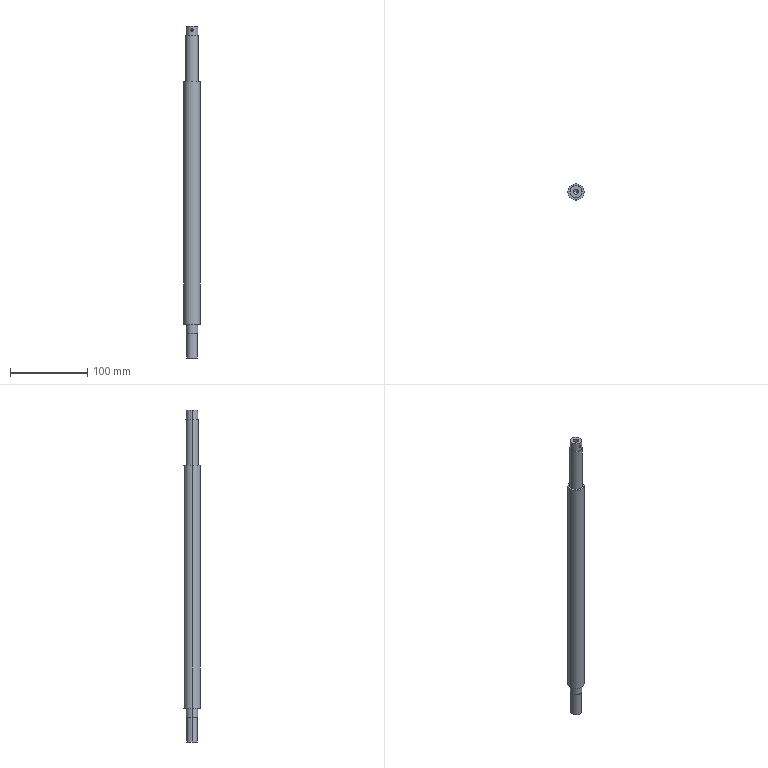Part | SolidWorks | features ICE 5, HoleWzd 2, 3DProfileFeature 1, Extrusion 1 | 1 solid | 28 faces | box 21 x 21 x 431 mm | volume 129224 mm3 | cylinder 16 | plane 10 | cone 2 | commonest cylinder face diameters 3.3 x4 15 x4 6.8 x2 14 x2 16 x2 21 x2
STEP:
#1=CARTESIAN_POINT('',(1.661,-7.314,6.663));
#2=VERTEX_POINT('',#1);
#3=CARTESIAN_POINT('',(-1.639,-7.319,6.663));
#4=VERTEX_POINT('',#3);
#5=CARTESIAN_POINT('',(1.661,-7.314,6.663));
#6=CARTESIAN_POINT('',(1.661,-7.314,6.448));
#7=CARTESIAN_POINT('',(1.617,-7.324,6.23));
#8=CARTESIAN_POINT('',(1.494,-7.35,5.932));
#9=CARTESIAN_POINT('',(1.442,-7.36,5.836));
#10=CARTESIAN_POINT('',(1.322,-7.383,5.656));
#11=CARTESIAN_POINT('',(1.254,-7.395,5.573));
#12=CARTESIAN_POINT('',(1.102,-7.419,5.421));
#13=CARTESIAN_POINT('',(1.018,-7.431,5.352));
#14=CARTESIAN_POINT('',(0.8393,-7.453,5.232));
#15=CARTESIAN_POINT('',(0.7447,-7.464,5.182));
#16=CARTESIAN_POINT('',(0.4441,-7.49,5.057));
#17=CARTESIAN_POINT('',(0.2295,-7.5,5.014));
#18=CARTESIAN_POINT('',(-0.09721,-7.5,5.013));
#19=CARTESIAN_POINT('',(-0.2045,-7.498,5.024));
#20=CARTESIAN_POINT('',(-0.4162,-7.489,5.066));
#21=CARTESIAN_POINT('',(-0.5215,-7.483,5.098));
#22=CARTESIAN_POINT('',(-0.8203,-7.458,5.222));
#23=CARTESIAN_POINT('',(-1.004,-7.434,5.345));
#24=CARTESIAN_POINT('',(-1.307,-7.387,5.647));
#25=CARTESIAN_POINT('',(-1.43,-7.363,5.831));
#26=CARTESIAN_POINT('',(-1.554,-7.337,6.129));
#27=CARTESIAN_POINT('',(-1.586,-7.33,6.233));
#28=CARTESIAN_POINT('',(-1.629,-7.321,6.446));
#29=CARTESIAN_POINT('',(-1.639,-7.319,6.554));
#30=CARTESIAN_POINT('',(-1.639,-7.319,6.663));
#31=B_SPLINE_CURVE_WITH_KNOTS('',3,(#5,#6,#7,#8,#9,#10,#11,#12,#13,#14,#15,#16,#17,#18,#19,#20,#21,#22,#23,#24,#25,#26,#27,#28,#29,#30),.UNSPECIFIED.,.F.,.F.,(4,2,2,2,2,2,2,2,2,2,2,2,4),(0.005174,0.005821,0.006144,0.006468,0.006791,0.007114,0.007761,0.008084,0.008408,0.009054,0.009701,0.01002,0.01035),.UNSPECIFIED.);
#32=EDGE_CURVE('',#2,#4,#31,.T.);
#33=ORIENTED_EDGE('',*,*,#32,.F.);
#34=CARTESIAN_POINT('',(1.654,-2.97,6.663));
#35=VERTEX_POINT('',#34);
#36=CARTESIAN_POINT('',(1.639,7.502,6.663));
#37=DIRECTION('',(-0.001464,1.,0.));
#38=VECTOR('',#37,1000.);
#39=LINE('',#36,#38);
#40=EDGE_CURVE('',#2,#35,#39,.T.);
#41=ORIENTED_EDGE('',*,*,#40,.T.);
#42=CARTESIAN_POINT('',(-1.646,-2.975,6.663));
#43=VERTEX_POINT('',#42);
#44=CARTESIAN_POINT('',(-1.646,-2.975,6.663));
#45=CARTESIAN_POINT('',(-1.646,-2.975,6.552));
#46=CARTESIAN_POINT('',(-1.635,-2.981,6.444));
#47=CARTESIAN_POINT('',(-1.592,-3.005,6.231));
#48=CARTESIAN_POINT('',(-1.559,-3.022,6.125));
#49=CARTESIAN_POINT('',(-1.434,-3.084,5.827));
#50=CARTESIAN_POINT('',(-1.312,-3.141,5.647));
#51=CARTESIAN_POINT('',(-1.013,-3.25,5.347));
#52=CARTESIAN_POINT('',(-0.8316,-3.303,5.225));
#53=CARTESIAN_POINT('',(-0.5341,-3.359,5.1));
#54=CARTESIAN_POINT('',(-0.4283,-3.375,5.068));
#55=CARTESIAN_POINT('',(-0.2142,-3.395,5.024));
#56=CARTESIAN_POINT('',(-0.1059,-3.4,5.013));
#57=CARTESIAN_POINT('',(0.1137,-3.4,5.013));
#58=CARTESIAN_POINT('',(0.2247,-3.394,5.025));
#59=CARTESIAN_POINT('',(0.4383,-3.373,5.068));
#60=CARTESIAN_POINT('',(0.543,-3.358,5.1));
#61=CARTESIAN_POINT('',(0.7435,-3.319,5.184));
#62=CARTESIAN_POINT('',(0.8377,-3.296,5.235));
#63=CARTESIAN_POINT('',(1.015,-3.246,5.355));
#64=CARTESIAN_POINT('',(1.098,-3.219,5.423));
#65=CARTESIAN_POINT('',(1.323,-3.136,5.649));
#66=CARTESIAN_POINT('',(1.444,-3.079,5.83));
#67=CARTESIAN_POINT('',(1.609,-2.996,6.225));
#68=CARTESIAN_POINT('',(1.654,-2.97,6.445));
#69=CARTESIAN_POINT('',(1.654,-2.97,6.663));
#70=B_SPLINE_CURVE_WITH_KNOTS('',3,(#44,#45,#46,#47,#48,#49,#50,#51,#52,#53,#54,#55,#56,#57,#58,#59,#60,#61,#62,#63,#64,#65,#66,#67,#68,#69),.UNSPECIFIED.,.F.,.F.,(4,2,2,2,2,2,2,2,2,2,2,2,4),(0.,0.0003276,0.0006553,0.001311,0.001966,0.002293,0.002621,0.002949,0.003276,0.003604,0.003932,0.004587,0.005242),.UNSPECIFIED.);
#71=EDGE_CURVE('',#43,#35,#70,.T.);
#72=ORIENTED_EDGE('',*,*,#71,.F.);
#73=CARTESIAN_POINT('',(-1.661,7.498,6.663));
#74=DIRECTION('',(-0.001464,1.,0.));
#75=VECTOR('',#74,1000.);
#76=LINE('',#73,#75);
#77=EDGE_CURVE('',#4,#43,#76,.T.);
#78=ORIENTED_EDGE('',*,*,#77,.F.);
#79=EDGE_LOOP('',(#33,#41,#72,#78));
#80=FACE_OUTER_BOUND('',#79,.T.);
#81=CARTESIAN_POINT('',(-0.01098,7.5,6.663));
#82=DIRECTION('',(-0.001464,1.,0.));
#83=DIRECTION('',(-1.,-0.001464,0.));
#84=AXIS2_PLACEMENT_3D('',#81,#82,#83);
#85=CYLINDRICAL_SURFACE('',#84,1.65);
#86=ADVANCED_FACE('',(#80),#85,.F.);
#87=CARTESIAN_POINT('',(1.646,2.975,6.663));
#88=VERTEX_POINT('',#87);
#89=CARTESIAN_POINT('',(-1.654,2.97,6.663));
#90=VERTEX_POINT('',#89);
#91=CARTESIAN_POINT('',(1.646,2.975,6.663));
#92=CARTESIAN_POINT('',(1.646,2.975,6.554));
#93=CARTESIAN_POINT('',(1.635,2.981,6.443));
#94=CARTESIAN_POINT('',(1.591,3.005,6.23));
#95=CARTESIAN_POINT('',(1.559,3.022,6.126));
#96=CARTESIAN_POINT('',(1.434,3.084,5.826));
#97=CARTESIAN_POINT('',(1.312,3.141,5.647));
#98=CARTESIAN_POINT('',(1.087,3.223,5.422));
#99=CARTESIAN_POINT('',(1.005,3.249,5.354));
#100=CARTESIAN_POINT('',(0.8279,3.299,5.235));
#101=CARTESIAN_POINT('',(0.7318,3.322,5.183));
#102=CARTESIAN_POINT('',(0.4346,3.378,5.059));
#103=CARTESIAN_POINT('',(0.2144,3.4,5.014));
#104=CARTESIAN_POINT('',(-0.1129,3.4,5.013));
#105=CARTESIAN_POINT('',(-0.2233,3.394,5.024));
#106=CARTESIAN_POINT('',(-0.4382,3.373,5.068));
#107=CARTESIAN_POINT('',(-0.5418,3.358,5.099));
#108=CARTESIAN_POINT('',(-0.8413,3.301,5.225));
#109=CARTESIAN_POINT('',(-1.021,3.247,5.346));
#110=CARTESIAN_POINT('',(-1.248,3.164,5.573));
#111=CARTESIAN_POINT('',(-1.315,3.136,5.655));
#112=CARTESIAN_POINT('',(-1.433,3.084,5.831));
#113=CARTESIAN_POINT('',(-1.485,3.059,5.927));
#114=CARTESIAN_POINT('',(-1.568,3.017,6.125));
#115=CARTESIAN_POINT('',(-1.6,3.,6.228));
#116=CARTESIAN_POINT('',(-1.643,2.977,6.441));
#117=CARTESIAN_POINT('',(-1.654,2.97,6.553));
#118=CARTESIAN_POINT('',(-1.654,2.97,6.663));
#119=B_SPLINE_CURVE_WITH_KNOTS('',3,(#91,#92,#93,#94,#95,#96,#97,#98,#99,#100,#101,#102,#103,#104,#105,#106,#107,#108,#109,#110,#111,#112,#113,#114,#115,#116,#117,#118),.UNSPECIFIED.,.F.,.F.,(4,2,2,2,2,2,2,2,2,2,2,2,2,4),(0.005242,0.005569,0.005896,0.006551,0.006878,0.007205,0.007859,0.008186,0.008514,0.009168,0.009495,0.009822,0.01015,0.01048),.UNSPECIFIED.);
#120=EDGE_CURVE('',#88,#90,#119,.T.);
#121=ORIENTED_EDGE('',*,*,#120,.F.);
#122=CARTESIAN_POINT('',(1.639,7.319,6.663));
#123=VERTEX_POINT('',#122);
#124=CARTESIAN_POINT('',(1.639,7.502,6.663));
#125=DIRECTION('',(-0.001464,1.,0.));
#126=VECTOR('',#125,1000.);
#127=LINE('',#124,#126);
#128=EDGE_CURVE('',#88,#123,#127,.T.);
#129=ORIENTED_EDGE('',*,*,#128,.T.);
#130=CARTESIAN_POINT('',(-1.661,7.314,6.663));
#131=VERTEX_POINT('',#130);
#132=CARTESIAN_POINT('',(-1.661,7.314,6.663));
#133=CARTESIAN_POINT('',(-1.661,7.314,6.554));
#134=CARTESIAN_POINT('',(-1.65,7.316,6.447));
#135=CARTESIAN_POINT('',(-1.608,7.326,6.235));
#136=CARTESIAN_POINT('',(-1.576,7.333,6.13));
#137=CARTESIAN_POINT('',(-1.493,7.35,5.931));
#138=CARTESIAN_POINT('',(-1.442,7.36,5.836));
#139=CARTESIAN_POINT('',(-1.323,7.383,5.657));
#140=CARTESIAN_POINT('',(-1.253,7.395,5.572));
#141=CARTESIAN_POINT('',(-1.026,7.431,5.345));
#142=CARTESIAN_POINT('',(-0.8421,7.455,5.222));
#143=CARTESIAN_POINT('',(-0.4452,7.489,5.057));
#144=CARTESIAN_POINT('',(-0.2276,7.5,5.014));
#145=CARTESIAN_POINT('',(0.09636,7.5,5.013));
#146=CARTESIAN_POINT('',(0.2061,7.498,5.024));
#147=CARTESIAN_POINT('',(0.418,7.489,5.067));
#148=CARTESIAN_POINT('',(0.521,7.483,5.098));
#149=CARTESIAN_POINT('',(0.8214,7.458,5.222));
#150=CARTESIAN_POINT('',(1.003,7.434,5.344));
#151=CARTESIAN_POINT('',(1.233,7.398,5.574));
#152=CARTESIAN_POINT('',(1.301,7.387,5.656));
#153=CARTESIAN_POINT('',(1.42,7.365,5.835));
#154=CARTESIAN_POINT('',(1.472,7.354,5.932));
#155=CARTESIAN_POINT('',(1.555,7.337,6.131));
#156=CARTESIAN_POINT('',(1.586,7.33,6.234));
#157=CARTESIAN_POINT('',(1.628,7.321,6.446));
#158=CARTESIAN_POINT('',(1.639,7.319,6.556));
#159=CARTESIAN_POINT('',(1.639,7.319,6.663));
#160=B_SPLINE_CURVE_WITH_KNOTS('',3,(#132,#133,#134,#135,#136,#137,#138,#139,#140,#141,#142,#143,#144,#145,#146,#147,#148,#149,#150,#151,#152,#153,#154,#155,#156,#157,#158,#159),.UNSPECIFIED.,.F.,.F.,(4,2,2,2,2,2,2,2,2,2,2,2,2,4),(0.,0.0003234,0.0006468,0.0009702,0.001294,0.00194,0.002587,0.002911,0.003234,0.003881,0.004204,0.004528,0.004851,0.005174),.UNSPECIFIED.);
#161=EDGE_CURVE('',#131,#123,#160,.T.);
#162=ORIENTED_EDGE('',*,*,#161,.F.);
#163=CARTESIAN_POINT('',(-1.661,7.498,6.663));
#164=DIRECTION('',(-0.001464,1.,0.));
#165=VECTOR('',#164,1000.);
#166=LINE('',#163,#165);
#167=EDGE_CURVE('',#90,#131,#166,.T.);
#168=ORIENTED_EDGE('',*,*,#167,.F.);
#169=EDGE_LOOP('',(#121,#129,#162,#168));
#170=FACE_OUTER_BOUND('',#169,.T.);
#171=CARTESIAN_POINT('',(-0.01098,7.5,6.663));
#172=DIRECTION('',(-0.001464,1.,0.));
#173=DIRECTION('',(-1.,-0.001464,0.));
#174=AXIS2_PLACEMENT_3D('',#171,#172,#173);
#175=CYLINDRICAL_SURFACE('',#174,1.65);
#176=ADVANCED_FACE('',(#170),#175,.F.);
#177=ORIENTED_EDGE('',*,*,#71,.T.);
#178=CARTESIAN_POINT('',(1.654,-2.97,6.663));
#179=CARTESIAN_POINT('',(1.654,-2.97,6.773));
#180=CARTESIAN_POINT('',(1.643,-2.977,6.884));
#181=CARTESIAN_POINT('',(1.6,-3.,7.097));
#182=CARTESIAN_POINT('',(1.568,-3.017,7.201));
#183=CARTESIAN_POINT('',(1.443,-3.08,7.501));
#184=CARTESIAN_POINT('',(1.321,-3.137,7.68));
#185=CARTESIAN_POINT('',(1.096,-3.219,7.905));
#186=CARTESIAN_POINT('',(1.015,-3.246,7.973));
#187=CARTESIAN_POINT('',(0.8375,-3.297,8.092));
#188=CARTESIAN_POINT('',(0.7416,-3.32,8.144));
#189=CARTESIAN_POINT('',(0.4444,-3.377,8.268));
#190=CARTESIAN_POINT('',(0.2244,-3.4,8.313));
#191=CARTESIAN_POINT('',(-0.1029,-3.4,8.314));
#192=CARTESIAN_POINT('',(-0.2134,-3.395,8.303));
#193=CARTESIAN_POINT('',(-0.4284,-3.375,8.259));
#194=CARTESIAN_POINT('',(-0.5319,-3.36,8.227));
#195=CARTESIAN_POINT('',(-0.8317,-3.303,8.102));
#196=CARTESIAN_POINT('',(-1.012,-3.25,7.981));
#197=CARTESIAN_POINT('',(-1.238,-3.167,7.754));
#198=CARTESIAN_POINT('',(-1.306,-3.14,7.672));
#199=CARTESIAN_POINT('',(-1.424,-3.088,7.496));
#200=CARTESIAN_POINT('',(-1.476,-3.063,7.4));
#201=CARTESIAN_POINT('',(-1.559,-3.022,7.201));
#202=CARTESIAN_POINT('',(-1.591,-3.005,7.099));
#203=CARTESIAN_POINT('',(-1.634,-2.982,6.885));
#204=CARTESIAN_POINT('',(-1.646,-2.975,6.774));
#205=CARTESIAN_POINT('',(-1.646,-2.975,6.663));
#206=B_SPLINE_CURVE_WITH_KNOTS('',3,(#178,#179,#180,#181,#182,#183,#184,#185,#186,#187,#188,#189,#190,#191,#192,#193,#194,#195,#196,#197,#198,#199,#200,#201,#202,#203,#204,#205),.UNSPECIFIED.,.F.,.F.,(4,2,2,2,2,2,2,2,2,2,2,2,2,4),(0.005242,0.005569,0.005896,0.006551,0.006878,0.007205,0.007859,0.008186,0.008514,0.009168,0.009495,0.009822,0.01015,0.01048),.UNSPECIFIED.);
#207=EDGE_CURVE('',#35,#43,#206,.T.);
#208=ORIENTED_EDGE('',*,*,#207,.T.);
#209=EDGE_LOOP('',(#177,#208));
#210=FACE_BOUND('',#209,.T.);
#211=CARTESIAN_POINT('',(-3.4,0.,-7.75));
#212=VERTEX_POINT('',#211);
#213=CARTESIAN_POINT('',(3.4,0.,-7.75));
#214=VERTEX_POINT('',#213);
#215=CARTESIAN_POINT('',(0.,0.,-7.75));
#216=DIRECTION('',(0.,0.,1.));
#217=DIRECTION('',(1.,0.,0.));
#218=AXIS2_PLACEMENT_3D('',#215,#216,#217);
#219=CIRCLE('',#218,3.4);
#220=EDGE_CURVE('',#212,#214,#219,.T.);
#221=ORIENTED_EDGE('',*,*,#220,.F.);
#222=CARTESIAN_POINT('',(-3.4,0.,12.));
#223=VERTEX_POINT('',#222);
#224=CARTESIAN_POINT('',(-3.4,0.,12.));
#225=DIRECTION('',(0.,0.,1.));
#226=VECTOR('',#225,1000.);
#227=LINE('',#224,#226);
#228=EDGE_CURVE('',#212,#223,#227,.T.);
#229=ORIENTED_EDGE('',*,*,#228,.T.);
#230=CARTESIAN_POINT('',(3.4,0.,12.));
#231=VERTEX_POINT('',#230);
#232=CARTESIAN_POINT('',(0.,0.,12.));
#233=DIRECTION('',(0.,0.,1.));
#234=DIRECTION('',(1.,0.,0.));
#235=AXIS2_PLACEMENT_3D('',#232,#233,#234);
#236=CIRCLE('',#235,3.4);
#237=EDGE_CURVE('',#223,#231,#236,.T.);
#238=ORIENTED_EDGE('',*,*,#237,.T.);
#239=CARTESIAN_POINT('',(3.4,0.,12.));
#240=DIRECTION('',(0.,0.,1.));
#241=VECTOR('',#240,1000.);
#242=LINE('',#239,#241);
#243=EDGE_CURVE('',#214,#231,#242,.T.);
#244=ORIENTED_EDGE('',*,*,#243,.F.);
#245=EDGE_LOOP('',(#221,#229,#238,#244));
#246=FACE_OUTER_BOUND('',#245,.T.);
#247=CARTESIAN_POINT('',(0.,0.,12.));
#248=DIRECTION('',(0.,0.,1.));
#249=DIRECTION('',(1.,0.,0.));
#250=AXIS2_PLACEMENT_3D('',#247,#248,#249);
#251=CYLINDRICAL_SURFACE('',#250,3.4);
#252=ADVANCED_FACE('',(#210,#246),#251,.F.);
#253=CARTESIAN_POINT('',(0.,0.,-9.793));
#254=VERTEX_POINT('',#253);
#255=CARTESIAN_POINT('',(3.4,0.,-7.75));
#256=DIRECTION('',(0.8572,0.,0.515));
#257=VECTOR('',#256,1000.);
#258=LINE('',#255,#257);
#259=EDGE_CURVE('',#254,#214,#258,.T.);
#260=ORIENTED_EDGE('',*,*,#259,.F.);
#261=CARTESIAN_POINT('',(-3.4,0.,-7.75));
#262=DIRECTION('',(-0.8572,0.,0.515));
#263=VECTOR('',#262,1000.);
#264=LINE('',#261,#263);
#265=EDGE_CURVE('',#254,#212,#264,.T.);
#266=ORIENTED_EDGE('',*,*,#265,.T.);
#267=ORIENTED_EDGE('',*,*,#220,.T.);
#268=EDGE_LOOP('',(#260,#266,#267));
#269=FACE_OUTER_BOUND('',#268,.T.);
#270=CARTESIAN_POINT('',(0.,0.,-7.75));
#271=DIRECTION('',(0.,0.,1.));
#272=DIRECTION('',(1.,0.,0.));
#273=AXIS2_PLACEMENT_3D('',#270,#271,#272);
#274=CONICAL_SURFACE('',#273,3.4,1.03);
#275=ADVANCED_FACE('',(#269),#274,.F.);
#276=CARTESIAN_POINT('',(-7.,0.,-419.));
#277=VERTEX_POINT('',#276);
#278=CARTESIAN_POINT('',(-2.354,6.592,-419.));
#279=VERTEX_POINT('',#278);
#280=CARTESIAN_POINT('',(0.,0.,-419.));
#281=DIRECTION('',(0.,0.,-1.));
#282=DIRECTION('',(-1.,0.,0.));
#283=AXIS2_PLACEMENT_3D('',#280,#281,#282);
#284=CIRCLE('',#283,7.);
#285=EDGE_CURVE('',#277,#279,#284,.T.);
#286=ORIENTED_EDGE('',*,*,#285,.F.);
#287=CARTESIAN_POINT('',(-7.,0.,-387.));
#288=VERTEX_POINT('',#287);
#289=CARTESIAN_POINT('',(-7.,0.,-419.));
#290=DIRECTION('',(0.,0.,1.));
#291=VECTOR('',#290,1000.);
#292=LINE('',#289,#291);
#293=EDGE_CURVE('',#277,#288,#292,.T.);
#294=ORIENTED_EDGE('',*,*,#293,.T.);
#295=CARTESIAN_POINT('',(7.,0.,-387.));
#296=VERTEX_POINT('',#295);
#297=CARTESIAN_POINT('',(0.,0.,-387.));
#298=DIRECTION('',(0.,0.,-1.));
#299=DIRECTION('',(-1.,0.,0.));
#300=AXIS2_PLACEMENT_3D('',#297,#298,#299);
#301=CIRCLE('',#300,7.);
#302=EDGE_CURVE('',#288,#296,#301,.T.);
#303=ORIENTED_EDGE('',*,*,#302,.T.);
#304=CARTESIAN_POINT('',(7.,0.,-419.));
#305=VERTEX_POINT('',#304);
#306=CARTESIAN_POINT('',(7.,0.,-419.));
#307=DIRECTION('',(0.,0.,1.));
#308=VECTOR('',#307,1000.);
#309=LINE('',#306,#308);
#310=EDGE_CURVE('',#305,#296,#309,.T.);
#311=ORIENTED_EDGE('',*,*,#310,.F.);
#312=CARTESIAN_POINT('',(2.354,6.592,-419.));
#313=VERTEX_POINT('',#312);
#314=CARTESIAN_POINT('',(0.,0.,-419.));
#315=DIRECTION('',(0.,0.,-1.));
#316=DIRECTION('',(-1.,0.,0.));
#317=AXIS2_PLACEMENT_3D('',#314,#315,#316);
#318=CIRCLE('',#317,7.);
#319=EDGE_CURVE('',#313,#305,#318,.T.);
#320=ORIENTED_EDGE('',*,*,#319,.F.);
#321=CARTESIAN_POINT('',(2.354,6.592,-389.));
#322=VERTEX_POINT('',#321);
#323=CARTESIAN_POINT('',(2.354,6.592,-419.));
#324=DIRECTION('',(0.,0.,1.));
#325=VECTOR('',#324,1000.);
#326=LINE('',#323,#325);
#327=EDGE_CURVE('',#313,#322,#326,.T.);
#328=ORIENTED_EDGE('',*,*,#327,.T.);
#329=CARTESIAN_POINT('',(-2.354,6.592,-389.));
#330=VERTEX_POINT('',#329);
#331=CARTESIAN_POINT('',(0.,0.,-389.));
#332=DIRECTION('',(0.,0.,1.));
#333=DIRECTION('',(1.,0.,0.));
#334=AXIS2_PLACEMENT_3D('',#331,#332,#333);
#335=CIRCLE('',#334,7.);
#336=EDGE_CURVE('',#322,#330,#335,.T.);
#337=ORIENTED_EDGE('',*,*,#336,.T.);
#338=CARTESIAN_POINT('',(-2.354,6.592,-419.));
#339=DIRECTION('',(0.,0.,-1.));
#340=VECTOR('',#339,1000.);
#341=LINE('',#338,#340);
#342=EDGE_CURVE('',#330,#279,#341,.T.);
#343=ORIENTED_EDGE('',*,*,#342,.T.);
#344=EDGE_LOOP('',(#286,#294,#303,#311,#320,#328,#337,#343));
#345=FACE_OUTER_BOUND('',#344,.T.);
#346=CARTESIAN_POINT('',(0.,0.,-419.));
#347=DIRECTION('',(0.,0.,1.));
#348=DIRECTION('',(1.,0.,0.));
#349=AXIS2_PLACEMENT_3D('',#346,#347,#348);
#350=CYLINDRICAL_SURFACE('',#349,7.);
#351=ADVANCED_FACE('',(#345),#350,.T.);
#352=CARTESIAN_POINT('',(-7.5,0.,-387.));
#353=VERTEX_POINT('',#352);
#354=CARTESIAN_POINT('',(7.5,0.,-387.));
#355=VERTEX_POINT('',#354);
#356=CARTESIAN_POINT('',(0.,0.,-387.));
#357=DIRECTION('',(0.,0.,-1.));
#358=DIRECTION('',(-1.,0.,0.));
#359=AXIS2_PLACEMENT_3D('',#356,#357,#358);
#360=CIRCLE('',#359,7.5);
#361=EDGE_CURVE('',#353,#355,#360,.T.);
#362=ORIENTED_EDGE('',*,*,#361,.F.);
#363=CARTESIAN_POINT('',(-7.5,0.,-375.));
#364=VERTEX_POINT('',#363);
#365=CARTESIAN_POINT('',(-7.5,0.,-387.));
#366=DIRECTION('',(0.,0.,1.));
#367=VECTOR('',#366,1000.);
#368=LINE('',#365,#367);
#369=EDGE_CURVE('',#353,#364,#368,.T.);
#370=ORIENTED_EDGE('',*,*,#369,.T.);
#371=CARTESIAN_POINT('',(7.5,0.,-375.));
#372=VERTEX_POINT('',#371);
#373=CARTESIAN_POINT('',(0.,0.,-375.));
#374=DIRECTION('',(0.,0.,-1.));
#375=DIRECTION('',(-1.,0.,0.));
#376=AXIS2_PLACEMENT_3D('',#373,#374,#375);
#377=CIRCLE('',#376,7.5);
#378=EDGE_CURVE('',#364,#372,#377,.T.);
#379=ORIENTED_EDGE('',*,*,#378,.T.);
#380=CARTESIAN_POINT('',(7.5,0.,-387.));
#381=DIRECTION('',(0.,0.,1.));
#382=VECTOR('',#381,1000.);
#383=LINE('',#380,#382);
#384=EDGE_CURVE('',#355,#372,#383,.T.);
#385=ORIENTED_EDGE('',*,*,#384,.F.);
#386=EDGE_LOOP('',(#362,#370,#379,#385));
#387=FACE_OUTER_BOUND('',#386,.T.);
#388=CARTESIAN_POINT('',(0.,0.,-387.));
#389=DIRECTION('',(0.,0.,1.));
#390=DIRECTION('',(1.,0.,0.));
#391=AXIS2_PLACEMENT_3D('',#388,#389,#390);
#392=CYLINDRICAL_SURFACE('',#391,7.5);
#393=ADVANCED_FACE('',(#387),#392,.T.);
#394=CARTESIAN_POINT('',(-10.5,0.,-375.));
#395=VERTEX_POINT('',#394);
#396=CARTESIAN_POINT('',(10.5,0.,-375.));
#397=VERTEX_POINT('',#396);
#398=CARTESIAN_POINT('',(0.,0.,-375.));
#399=DIRECTION('',(0.,0.,-1.));
#400=DIRECTION('',(-1.,0.,0.));
#401=AXIS2_PLACEMENT_3D('',#398,#399,#400);
#402=CIRCLE('',#401,10.5);
#403=EDGE_CURVE('',#395,#397,#402,.T.);
#404=ORIENTED_EDGE('',*,*,#403,.F.);
#405=CARTESIAN_POINT('',(-10.5,0.,-60.));
#406=VERTEX_POINT('',#405);
#407=CARTESIAN_POINT('',(-10.5,0.,-375.));
#408=DIRECTION('',(0.,0.,1.));
#409=VECTOR('',#408,1000.);
#410=LINE('',#407,#409);
#411=EDGE_CURVE('',#395,#406,#410,.T.);
#412=ORIENTED_EDGE('',*,*,#411,.T.);
#413=CARTESIAN_POINT('',(10.5,0.,-60.));
#414=VERTEX_POINT('',#413);
#415=CARTESIAN_POINT('',(0.,0.,-60.));
#416=DIRECTION('',(0.,0.,-1.));
#417=DIRECTION('',(-1.,0.,0.));
#418=AXIS2_PLACEMENT_3D('',#415,#416,#417);
#419=CIRCLE('',#418,10.5);
#420=EDGE_CURVE('',#406,#414,#419,.T.);
#421=ORIENTED_EDGE('',*,*,#420,.T.);
#422=CARTESIAN_POINT('',(10.5,0.,-375.));
#423=DIRECTION('',(0.,0.,1.));
#424=VECTOR('',#423,1000.);
#425=LINE('',#422,#424);
#426=EDGE_CURVE('',#397,#414,#425,.T.);
#427=ORIENTED_EDGE('',*,*,#426,.F.);
#428=EDGE_LOOP('',(#404,#412,#421,#427));
#429=FACE_OUTER_BOUND('',#428,.T.);
#430=CARTESIAN_POINT('',(0.,0.,-375.));
#431=DIRECTION('',(0.,0.,1.));
#432=DIRECTION('',(1.,0.,0.));
#433=AXIS2_PLACEMENT_3D('',#430,#431,#432);
#434=CYLINDRICAL_SURFACE('',#433,10.5);
#435=ADVANCED_FACE('',(#429),#434,.T.);
#436=CARTESIAN_POINT('',(-8.,0.,-60.));
#437=VERTEX_POINT('',#436);
#438=CARTESIAN_POINT('',(8.,0.,-60.));
#439=VERTEX_POINT('',#438);
#440=CARTESIAN_POINT('',(0.,0.,-60.));
#441=DIRECTION('',(0.,0.,-1.));
#442=DIRECTION('',(-1.,0.,0.));
#443=AXIS2_PLACEMENT_3D('',#440,#441,#442);
#444=CIRCLE('',#443,8.);
#445=EDGE_CURVE('',#437,#439,#444,.T.);
#446=ORIENTED_EDGE('',*,*,#445,.F.);
#447=CARTESIAN_POINT('',(-8.,0.,0.));
#448=VERTEX_POINT('',#447);
#449=CARTESIAN_POINT('',(-8.,0.,-60.));
#450=DIRECTION('',(0.,0.,1.));
#451=VECTOR('',#450,1000.);
#452=LINE('',#449,#451);
#453=EDGE_CURVE('',#437,#448,#452,.T.);
#454=ORIENTED_EDGE('',*,*,#453,.T.);
#455=CARTESIAN_POINT('',(8.,0.,0.));
#456=VERTEX_POINT('',#455);
#457=CARTESIAN_POINT('',(0.,0.,0.));
#458=DIRECTION('',(0.,0.,-1.));
#459=DIRECTION('',(-1.,0.,0.));
#460=AXIS2_PLACEMENT_3D('',#457,#458,#459);
#461=CIRCLE('',#460,8.);
#462=EDGE_CURVE('',#448,#456,#461,.T.);
#463=ORIENTED_EDGE('',*,*,#462,.T.);
#464=CARTESIAN_POINT('',(8.,0.,-60.));
#465=DIRECTION('',(0.,0.,1.));
#466=VECTOR('',#465,1000.);
#467=LINE('',#464,#466);
#468=EDGE_CURVE('',#439,#456,#467,.T.);
#469=ORIENTED_EDGE('',*,*,#468,.F.);
#470=EDGE_LOOP('',(#446,#454,#463,#469));
#471=FACE_OUTER_BOUND('',#470,.T.);
#472=CARTESIAN_POINT('',(0.,0.,-60.));
#473=DIRECTION('',(0.,0.,1.));
#474=DIRECTION('',(1.,0.,0.));
#475=AXIS2_PLACEMENT_3D('',#472,#473,#474);
#476=CYLINDRICAL_SURFACE('',#475,8.);
#477=ADVANCED_FACE('',(#471),#476,.T.);
#478=ORIENTED_EDGE('',*,*,#161,.T.);
#479=CARTESIAN_POINT('',(1.639,7.319,6.663));
#480=CARTESIAN_POINT('',(1.639,7.319,6.879));
#481=CARTESIAN_POINT('',(1.596,7.329,7.097));
#482=CARTESIAN_POINT('',(1.472,7.354,7.395));
#483=CARTESIAN_POINT('',(1.421,7.364,7.491));
#484=CARTESIAN_POINT('',(1.301,7.387,7.671));
#485=CARTESIAN_POINT('',(1.233,7.398,7.753));
#486=CARTESIAN_POINT('',(1.081,7.422,7.906));
#487=CARTESIAN_POINT('',(0.9959,7.434,7.975));
#488=CARTESIAN_POINT('',(0.8174,7.456,8.094));
#489=CARTESIAN_POINT('',(0.7228,7.466,8.145));
#490=CARTESIAN_POINT('',(0.4222,7.491,8.27));
#491=CARTESIAN_POINT('',(0.2075,7.5,8.313));
#492=CARTESIAN_POINT('',(-0.1192,7.5,8.313));
#493=CARTESIAN_POINT('',(-0.2265,7.497,8.303));
#494=CARTESIAN_POINT('',(-0.4381,7.488,8.261));
#495=CARTESIAN_POINT('',(-0.5434,7.481,8.229));
#496=CARTESIAN_POINT('',(-0.8421,7.455,8.105));
#497=CARTESIAN_POINT('',(-1.025,7.431,7.982));
#498=CARTESIAN_POINT('',(-1.329,7.383,7.679));
#499=CARTESIAN_POINT('',(-1.451,7.359,7.496));
#500=CARTESIAN_POINT('',(-1.575,7.333,7.198));
#501=CARTESIAN_POINT('',(-1.607,7.326,7.093));
#502=CARTESIAN_POINT('',(-1.65,7.316,6.881));
#503=CARTESIAN_POINT('',(-1.661,7.314,6.773));
#504=CARTESIAN_POINT('',(-1.661,7.314,6.663));
#505=B_SPLINE_CURVE_WITH_KNOTS('',3,(#479,#480,#481,#482,#483,#484,#485,#486,#487,#488,#489,#490,#491,#492,#493,#494,#495,#496,#497,#498,#499,#500,#501,#502,#503,#504),.UNSPECIFIED.,.F.,.F.,(4,2,2,2,2,2,2,2,2,2,2,2,4),(0.005174,0.005821,0.006144,0.006468,0.006791,0.007114,0.007761,0.008084,0.008408,0.009054,0.009701,0.01002,0.01035),.UNSPECIFIED.);
#506=EDGE_CURVE('',#123,#131,#505,.T.);
#507=ORIENTED_EDGE('',*,*,#506,.T.);
#508=EDGE_LOOP('',(#478,#507));
#509=FACE_BOUND('',#508,.T.);
#510=CARTESIAN_POINT('',(7.5,0.,12.));
#511=VERTEX_POINT('',#510);
#512=CARTESIAN_POINT('',(-7.5,0.,12.));
#513=VERTEX_POINT('',#512);
#514=CARTESIAN_POINT('',(0.,0.,12.));
#515=DIRECTION('',(0.,0.,1.));
#516=DIRECTION('',(1.,0.,0.));
#517=AXIS2_PLACEMENT_3D('',#514,#515,#516);
#518=CIRCLE('',#517,7.5);
#519=EDGE_CURVE('',#511,#513,#518,.T.);
#520=ORIENTED_EDGE('',*,*,#519,.F.);
#521=CARTESIAN_POINT('',(7.5,0.,0.));
#522=VERTEX_POINT('',#521);
#523=CARTESIAN_POINT('',(7.5,0.,12.));
#524=DIRECTION('',(0.,0.,-1.));
#525=VECTOR('',#524,1000.);
#526=LINE('',#523,#525);
#527=EDGE_CURVE('',#511,#522,#526,.T.);
#528=ORIENTED_EDGE('',*,*,#527,.T.);
#529=CARTESIAN_POINT('',(-7.5,0.,0.));
#530=VERTEX_POINT('',#529);
#531=CARTESIAN_POINT('',(0.,0.,0.));
#532=DIRECTION('',(0.,0.,-1.));
#533=DIRECTION('',(-1.,0.,0.));
#534=AXIS2_PLACEMENT_3D('',#531,#532,#533);
#535=CIRCLE('',#534,7.5);
#536=EDGE_CURVE('',#530,#522,#535,.T.);
#537=ORIENTED_EDGE('',*,*,#536,.F.);
#538=CARTESIAN_POINT('',(-7.5,0.,12.));
#539=DIRECTION('',(0.,0.,-1.));
#540=VECTOR('',#539,1000.);
#541=LINE('',#538,#540);
#542=EDGE_CURVE('',#513,#530,#541,.T.);
#543=ORIENTED_EDGE('',*,*,#542,.F.);
#544=EDGE_LOOP('',(#520,#528,#537,#543));
#545=FACE_OUTER_BOUND('',#544,.T.);
#546=CARTESIAN_POINT('',(0.,0.,12.));
#547=DIRECTION('',(0.,0.,-1.));
#548=DIRECTION('',(-1.,0.,0.));
#549=AXIS2_PLACEMENT_3D('',#546,#547,#548);
#550=CYLINDRICAL_SURFACE('',#549,7.5);
#551=ADVANCED_FACE('',(#509,#545),#550,.T.);
#552=CARTESIAN_POINT('',(0.,0.,-387.));
#553=DIRECTION('',(0.,0.,-1.));
#554=DIRECTION('',(-1.,0.,0.));
#555=AXIS2_PLACEMENT_3D('',#552,#553,#554);
#556=CIRCLE('',#555,7.5);
#557=EDGE_CURVE('',#355,#353,#556,.T.);
#558=ORIENTED_EDGE('',*,*,#557,.T.);
#559=ORIENTED_EDGE('',*,*,#361,.T.);
#560=EDGE_LOOP('',(#558,#559));
#561=FACE_OUTER_BOUND('',#560,.T.);
#562=CARTESIAN_POINT('',(0.,0.,-387.));
#563=DIRECTION('',(0.,0.,-1.));
#564=DIRECTION('',(-1.,0.,0.));
#565=AXIS2_PLACEMENT_3D('',#562,#563,#564);
#566=CIRCLE('',#565,7.);
#567=EDGE_CURVE('',#296,#288,#566,.T.);
#568=ORIENTED_EDGE('',*,*,#567,.F.);
#569=ORIENTED_EDGE('',*,*,#302,.F.);
#570=EDGE_LOOP('',(#568,#569));
#571=FACE_BOUND('',#570,.T.);
#572=CARTESIAN_POINT('',(0.,0.,-387.));
#573=DIRECTION('',(0.,0.,-1.));
#574=DIRECTION('',(-1.,0.,0.));
#575=AXIS2_PLACEMENT_3D('',#572,#573,#574);
#576=PLANE('',#575);
#577=ADVANCED_FACE('',(#561,#571),#576,.T.);
#578=CARTESIAN_POINT('',(0.,0.,-375.));
#579=DIRECTION('',(0.,0.,-1.));
#580=DIRECTION('',(-1.,0.,0.));
#581=AXIS2_PLACEMENT_3D('',#578,#579,#580);
#582=CIRCLE('',#581,10.5);
#583=EDGE_CURVE('',#397,#395,#582,.T.);
#584=ORIENTED_EDGE('',*,*,#583,.T.);
#585=ORIENTED_EDGE('',*,*,#403,.T.);
#586=EDGE_LOOP('',(#584,#585));
#587=FACE_OUTER_BOUND('',#586,.T.);
#588=CARTESIAN_POINT('',(0.,0.,-375.));
#589=DIRECTION('',(0.,0.,-1.));
#590=DIRECTION('',(-1.,0.,0.));
#591=AXIS2_PLACEMENT_3D('',#588,#589,#590);
#592=CIRCLE('',#591,7.5);
#593=EDGE_CURVE('',#372,#364,#592,.T.);
#594=ORIENTED_EDGE('',*,*,#593,.F.);
#595=ORIENTED_EDGE('',*,*,#378,.F.);
#596=EDGE_LOOP('',(#594,#595));
#597=FACE_BOUND('',#596,.T.);
#598=CARTESIAN_POINT('',(0.,0.,-375.));
#599=DIRECTION('',(0.,0.,-1.));
#600=DIRECTION('',(-1.,0.,0.));
#601=AXIS2_PLACEMENT_3D('',#598,#599,#600);
#602=PLANE('',#601);
#603=ADVANCED_FACE('',(#587,#597),#602,.T.);
#604=ORIENTED_EDGE('',*,*,#527,.F.);
#605=CARTESIAN_POINT('',(0.,0.,12.));
#606=DIRECTION('',(0.,0.,1.));
#607=DIRECTION('',(1.,0.,0.));
#608=AXIS2_PLACEMENT_3D('',#605,#606,#607);
#609=CIRCLE('',#608,7.5);
#610=EDGE_CURVE('',#513,#511,#609,.T.);
#611=ORIENTED_EDGE('',*,*,#610,.F.);
#612=ORIENTED_EDGE('',*,*,#542,.T.);
#613=CARTESIAN_POINT('',(0.,0.,0.));
#614=DIRECTION('',(0.,0.,-1.));
#615=DIRECTION('',(-1.,0.,0.));
#616=AXIS2_PLACEMENT_3D('',#613,#614,#615);
#617=CIRCLE('',#616,7.5);
#618=EDGE_CURVE('',#522,#530,#617,.T.);
#619=ORIENTED_EDGE('',*,*,#618,.F.);
#620=EDGE_LOOP('',(#604,#611,#612,#619));
#621=FACE_OUTER_BOUND('',#620,.T.);
#622=CARTESIAN_POINT('',(-1.639,-7.319,6.663));
#623=CARTESIAN_POINT('',(-1.639,-7.319,6.773));
#624=CARTESIAN_POINT('',(-1.629,-7.321,6.88));
#625=CARTESIAN_POINT('',(-1.586,-7.33,7.092));
#626=CARTESIAN_POINT('',(-1.554,-7.337,7.197));
#627=CARTESIAN_POINT('',(-1.471,-7.354,7.396));
#628=CARTESIAN_POINT('',(-1.421,-7.364,7.491));
#629=CARTESIAN_POINT('',(-1.301,-7.387,7.67));
#630=CARTESIAN_POINT('',(-1.232,-7.399,7.755));
#631=CARTESIAN_POINT('',(-1.004,-7.434,7.982));
#632=CARTESIAN_POINT('',(-0.8202,-7.458,8.105));
#633=CARTESIAN_POINT('',(-0.4233,-7.491,8.27));
#634=CARTESIAN_POINT('',(-0.2057,-7.5,8.313));
#635=CARTESIAN_POINT('',(0.1183,-7.5,8.313));
#636=CARTESIAN_POINT('',(0.228,-7.497,8.303));
#637=CARTESIAN_POINT('',(0.4399,-7.488,8.26));
#638=CARTESIAN_POINT('',(0.5429,-7.481,8.229));
#639=CARTESIAN_POINT('',(0.8432,-7.455,8.105));
#640=CARTESIAN_POINT('',(1.025,-7.431,7.983));
#641=CARTESIAN_POINT('',(1.254,-7.395,7.753));
#642=CARTESIAN_POINT('',(1.322,-7.383,7.67));
#643=CARTESIAN_POINT('',(1.442,-7.36,7.492));
#644=CARTESIAN_POINT('',(1.494,-7.35,7.395));
#645=CARTESIAN_POINT('',(1.576,-7.333,7.196));
#646=CARTESIAN_POINT('',(1.607,-7.326,7.093));
#647=CARTESIAN_POINT('',(1.65,-7.316,6.881));
#648=CARTESIAN_POINT('',(1.661,-7.314,6.771));
#649=CARTESIAN_POINT('',(1.661,-7.314,6.663));
#650=B_SPLINE_CURVE_WITH_KNOTS('',3,(#622,#623,#624,#625,#626,#627,#628,#629,#630,#631,#632,#633,#634,#635,#636,#637,#638,#639,#640,#641,#642,#643,#644,#645,#646,#647,#648,#649),.UNSPECIFIED.,.F.,.F.,(4,2,2,2,2,2,2,2,2,2,2,2,2,4),(0.,0.0003234,0.0006468,0.0009702,0.001294,0.00194,0.002587,0.002911,0.003234,0.003881,0.004204,0.004528,0.004851,0.005174),.UNSPECIFIED.);
#651=EDGE_CURVE('',#4,#2,#650,.T.);
#652=ORIENTED_EDGE('',*,*,#651,.T.);
#653=ORIENTED_EDGE('',*,*,#32,.T.);
#654=EDGE_LOOP('',(#652,#653));
#655=FACE_BOUND('',#654,.T.);
#656=CARTESIAN_POINT('',(0.,0.,12.));
#657=DIRECTION('',(0.,0.,-1.));
#658=DIRECTION('',(-1.,0.,0.));
#659=AXIS2_PLACEMENT_3D('',#656,#657,#658);
#660=CYLINDRICAL_SURFACE('',#659,7.5);
#661=ADVANCED_FACE('',(#621,#655),#660,.T.);
#662=CARTESIAN_POINT('',(0.,0.,12.));
#663=DIRECTION('',(0.,0.,1.));
#664=DIRECTION('',(1.,0.,0.));
#665=AXIS2_PLACEMENT_3D('',#662,#663,#664);
#666=CIRCLE('',#665,3.4);
#667=EDGE_CURVE('',#231,#223,#666,.T.);
#668=ORIENTED_EDGE('',*,*,#667,.F.);
#669=ORIENTED_EDGE('',*,*,#237,.F.);
#670=EDGE_LOOP('',(#668,#669));
#671=FACE_BOUND('',#670,.T.);
#672=ORIENTED_EDGE('',*,*,#610,.T.);
#673=ORIENTED_EDGE('',*,*,#519,.T.);
#674=EDGE_LOOP('',(#672,#673));
#675=FACE_OUTER_BOUND('',#674,.T.);
#676=CARTESIAN_POINT('',(0.,0.,12.));
#677=DIRECTION('',(0.,0.,1.));
#678=DIRECTION('',(1.,0.,0.));
#679=AXIS2_PLACEMENT_3D('',#676,#677,#678);
#680=PLANE('',#679);
#681=ADVANCED_FACE('',(#671,#675),#680,.T.);
#682=CARTESIAN_POINT('',(0.,0.,0.));
#683=DIRECTION('',(0.,0.,-1.));
#684=DIRECTION('',(-1.,0.,0.));
#685=AXIS2_PLACEMENT_3D('',#682,#683,#684);
#686=CIRCLE('',#685,8.);
#687=EDGE_CURVE('',#456,#448,#686,.T.);
#688=ORIENTED_EDGE('',*,*,#687,.F.);
#689=ORIENTED_EDGE('',*,*,#462,.F.);
#690=EDGE_LOOP('',(#688,#689));
#691=FACE_OUTER_BOUND('',#690,.T.);
#692=ORIENTED_EDGE('',*,*,#536,.T.);
#693=ORIENTED_EDGE('',*,*,#618,.T.);
#694=EDGE_LOOP('',(#692,#693));
#695=FACE_BOUND('',#694,.T.);
#696=CARTESIAN_POINT('',(0.,0.,0.));
#697=DIRECTION('',(0.,0.,-1.));
#698=DIRECTION('',(-1.,0.,0.));
#699=AXIS2_PLACEMENT_3D('',#696,#697,#698);
#700=PLANE('',#699);
#701=ADVANCED_FACE('',(#691,#695),#700,.F.);
#702=ORIENTED_EDGE('',*,*,#453,.F.);
#703=CARTESIAN_POINT('',(0.,0.,-60.));
#704=DIRECTION('',(0.,0.,-1.));
#705=DIRECTION('',(-1.,0.,0.));
#706=AXIS2_PLACEMENT_3D('',#703,#704,#705);
#707=CIRCLE('',#706,8.);
#708=EDGE_CURVE('',#439,#437,#707,.T.);
#709=ORIENTED_EDGE('',*,*,#708,.F.);
#710=ORIENTED_EDGE('',*,*,#468,.T.);
#711=ORIENTED_EDGE('',*,*,#687,.T.);
#712=EDGE_LOOP('',(#702,#709,#710,#711));
#713=FACE_OUTER_BOUND('',#712,.T.);
#714=CARTESIAN_POINT('',(0.,0.,-60.));
#715=DIRECTION('',(0.,0.,1.));
#716=DIRECTION('',(1.,0.,0.));
#717=AXIS2_PLACEMENT_3D('',#714,#715,#716);
#718=CYLINDRICAL_SURFACE('',#717,8.);
#719=ADVANCED_FACE('',(#713),#718,.T.);
#720=CARTESIAN_POINT('',(0.,0.,-60.));
#721=DIRECTION('',(0.,0.,-1.));
#722=DIRECTION('',(-1.,0.,0.));
#723=AXIS2_PLACEMENT_3D('',#720,#721,#722);
#724=CIRCLE('',#723,10.5);
#725=EDGE_CURVE('',#414,#406,#724,.T.);
#726=ORIENTED_EDGE('',*,*,#725,.F.);
#727=ORIENTED_EDGE('',*,*,#420,.F.);
#728=EDGE_LOOP('',(#726,#727));
#729=FACE_OUTER_BOUND('',#728,.T.);
#730=ORIENTED_EDGE('',*,*,#708,.T.);
#731=ORIENTED_EDGE('',*,*,#445,.T.);
#732=EDGE_LOOP('',(#730,#731));
#733=FACE_BOUND('',#732,.T.);
#734=CARTESIAN_POINT('',(0.,0.,-60.));
#735=DIRECTION('',(0.,0.,-1.));
#736=DIRECTION('',(-1.,0.,0.));
#737=AXIS2_PLACEMENT_3D('',#734,#735,#736);
#738=PLANE('',#737);
#739=ADVANCED_FACE('',(#729,#733),#738,.F.);
#740=ORIENTED_EDGE('',*,*,#411,.F.);
#741=ORIENTED_EDGE('',*,*,#583,.F.);
#742=ORIENTED_EDGE('',*,*,#426,.T.);
#743=ORIENTED_EDGE('',*,*,#725,.T.);
#744=EDGE_LOOP('',(#740,#741,#742,#743));
#745=FACE_OUTER_BOUND('',#744,.T.);
#746=CARTESIAN_POINT('',(0.,0.,-375.));
#747=DIRECTION('',(0.,0.,1.));
#748=DIRECTION('',(1.,0.,0.));
#749=AXIS2_PLACEMENT_3D('',#746,#747,#748);
#750=CYLINDRICAL_SURFACE('',#749,10.5);
#751=ADVANCED_FACE('',(#745),#750,.T.);
#752=ORIENTED_EDGE('',*,*,#369,.F.);
#753=ORIENTED_EDGE('',*,*,#557,.F.);
#754=ORIENTED_EDGE('',*,*,#384,.T.);
#755=ORIENTED_EDGE('',*,*,#593,.T.);
#756=EDGE_LOOP('',(#752,#753,#754,#755));
#757=FACE_OUTER_BOUND('',#756,.T.);
#758=CARTESIAN_POINT('',(0.,0.,-387.));
#759=DIRECTION('',(0.,0.,1.));
#760=DIRECTION('',(1.,0.,0.));
#761=AXIS2_PLACEMENT_3D('',#758,#759,#760);
#762=CYLINDRICAL_SURFACE('',#761,7.5);
#763=ADVANCED_FACE('',(#757),#762,.T.);
#764=ORIENTED_EDGE('',*,*,#293,.F.);
#765=CARTESIAN_POINT('',(0.,0.,-419.));
#766=DIRECTION('',(0.,0.,-1.));
#767=DIRECTION('',(-1.,0.,0.));
#768=AXIS2_PLACEMENT_3D('',#765,#766,#767);
#769=CIRCLE('',#768,7.);
#770=EDGE_CURVE('',#305,#277,#769,.T.);
#771=ORIENTED_EDGE('',*,*,#770,.F.);
#772=ORIENTED_EDGE('',*,*,#310,.T.);
#773=ORIENTED_EDGE('',*,*,#567,.T.);
#774=EDGE_LOOP('',(#764,#771,#772,#773));
#775=FACE_OUTER_BOUND('',#774,.T.);
#776=CARTESIAN_POINT('',(0.,0.,-419.));
#777=DIRECTION('',(0.,0.,1.));
#778=DIRECTION('',(1.,0.,0.));
#779=AXIS2_PLACEMENT_3D('',#776,#777,#778);
#780=CYLINDRICAL_SURFACE('',#779,7.);
#781=ADVANCED_FACE('',(#775),#780,.T.);
#782=CARTESIAN_POINT('',(2.354,4.758,-419.));
#783=VERTEX_POINT('',#782);
#784=CARTESIAN_POINT('',(2.354,0.,-419.));
#785=DIRECTION('',(0.,-1.,0.));
#786=VECTOR('',#785,1000.);
#787=LINE('',#784,#786);
#788=EDGE_CURVE('',#313,#783,#787,.T.);
#789=ORIENTED_EDGE('',*,*,#788,.F.);
#790=ORIENTED_EDGE('',*,*,#319,.T.);
#791=ORIENTED_EDGE('',*,*,#770,.T.);
#792=ORIENTED_EDGE('',*,*,#285,.T.);
#793=CARTESIAN_POINT('',(-2.354,4.758,-419.));
#794=VERTEX_POINT('',#793);
#795=CARTESIAN_POINT('',(-2.354,9.242,-419.));
#796=DIRECTION('',(0.,1.,0.));
#797=VECTOR('',#796,1000.);
#798=LINE('',#795,#797);
#799=EDGE_CURVE('',#794,#279,#798,.T.);
#800=ORIENTED_EDGE('',*,*,#799,.F.);
#801=CARTESIAN_POINT('',(-2.354,4.758,-419.));
#802=DIRECTION('',(-1.,0.,0.));
#803=VECTOR('',#802,1000.);
#804=LINE('',#801,#803);
#805=EDGE_CURVE('',#783,#794,#804,.T.);
#806=ORIENTED_EDGE('',*,*,#805,.F.);
#807=EDGE_LOOP('',(#789,#790,#791,#792,#800,#806));
#808=FACE_OUTER_BOUND('',#807,.T.);
#809=CARTESIAN_POINT('',(0.,0.,-419.));
#810=DIRECTION('',(0.,0.,-1.));
#811=DIRECTION('',(-1.,0.,0.));
#812=AXIS2_PLACEMENT_3D('',#809,#810,#811);
#813=PLANE('',#812);
#814=ADVANCED_FACE('',(#808),#813,.T.);
#815=CARTESIAN_POINT('',(2.354,4.758,-389.));
#816=VERTEX_POINT('',#815);
#817=CARTESIAN_POINT('',(2.354,9.242,-389.));
#818=DIRECTION('',(0.,-1.,0.));
#819=VECTOR('',#818,1000.);
#820=LINE('',#817,#819);
#821=EDGE_CURVE('',#322,#816,#820,.T.);
#822=ORIENTED_EDGE('',*,*,#821,.T.);
#823=CARTESIAN_POINT('',(-2.354,4.758,-389.));
#824=VERTEX_POINT('',#823);
#825=CARTESIAN_POINT('',(-2.354,4.758,-389.));
#826=DIRECTION('',(-1.,0.,0.));
#827=VECTOR('',#826,1000.);
#828=LINE('',#825,#827);
#829=EDGE_CURVE('',#816,#824,#828,.T.);
#830=ORIENTED_EDGE('',*,*,#829,.T.);
#831=CARTESIAN_POINT('',(-2.354,9.242,-389.));
#832=DIRECTION('',(0.,1.,0.));
#833=VECTOR('',#832,1000.);
#834=LINE('',#831,#833);
#835=EDGE_CURVE('',#824,#330,#834,.T.);
#836=ORIENTED_EDGE('',*,*,#835,.T.);
#837=ORIENTED_EDGE('',*,*,#336,.F.);
#838=EDGE_LOOP('',(#822,#830,#836,#837));
#839=FACE_OUTER_BOUND('',#838,.T.);
#840=CARTESIAN_POINT('',(0.,0.,-389.));
#841=DIRECTION('',(0.,0.,1.));
#842=DIRECTION('',(1.,0.,0.));
#843=AXIS2_PLACEMENT_3D('',#840,#841,#842);
#844=PLANE('',#843);
#845=ADVANCED_FACE('',(#839),#844,.F.);
#846=ORIENTED_EDGE('',*,*,#788,.T.);
#847=CARTESIAN_POINT('',(2.354,4.758,-389.));
#848=DIRECTION('',(0.,0.,-1.));
#849=VECTOR('',#848,1000.);
#850=LINE('',#847,#849);
#851=EDGE_CURVE('',#816,#783,#850,.T.);
#852=ORIENTED_EDGE('',*,*,#851,.F.);
#853=ORIENTED_EDGE('',*,*,#821,.F.);
#854=ORIENTED_EDGE('',*,*,#327,.F.);
#855=EDGE_LOOP('',(#846,#852,#853,#854));
#856=FACE_OUTER_BOUND('',#855,.T.);
#857=CARTESIAN_POINT('',(2.354,9.242,-389.));
#858=DIRECTION('',(1.,0.,0.));
#859=DIRECTION('',(0.,0.,-1.));
#860=AXIS2_PLACEMENT_3D('',#857,#858,#859);
#861=PLANE('',#860);
#862=ADVANCED_FACE('',(#856),#861,.F.);
#863=ORIENTED_EDGE('',*,*,#835,.F.);
#864=CARTESIAN_POINT('',(-2.354,4.758,-389.));
#865=DIRECTION('',(0.,0.,-1.));
#866=VECTOR('',#865,1000.);
#867=LINE('',#864,#866);
#868=EDGE_CURVE('',#824,#794,#867,.T.);
#869=ORIENTED_EDGE('',*,*,#868,.T.);
#870=ORIENTED_EDGE('',*,*,#799,.T.);
#871=ORIENTED_EDGE('',*,*,#342,.F.);
#872=EDGE_LOOP('',(#863,#869,#870,#871));
#873=FACE_OUTER_BOUND('',#872,.T.);
#874=CARTESIAN_POINT('',(-2.354,9.242,-389.));
#875=DIRECTION('',(-1.,0.,0.));
#876=DIRECTION('',(0.,0.,1.));
#877=AXIS2_PLACEMENT_3D('',#874,#875,#876);
#878=PLANE('',#877);
#879=ADVANCED_FACE('',(#873),#878,.F.);
#880=ORIENTED_EDGE('',*,*,#805,.T.);
#881=ORIENTED_EDGE('',*,*,#868,.F.);
#882=ORIENTED_EDGE('',*,*,#829,.F.);
#883=ORIENTED_EDGE('',*,*,#851,.T.);
#884=EDGE_LOOP('',(#880,#881,#882,#883));
#885=FACE_OUTER_BOUND('',#884,.T.);
#886=CARTESIAN_POINT('',(-2.354,4.758,-389.));
#887=DIRECTION('',(0.,-1.,0.));
#888=DIRECTION('',(0.,0.,-1.));
#889=AXIS2_PLACEMENT_3D('',#886,#887,#888);
#890=PLANE('',#889);
#891=ADVANCED_FACE('',(#885),#890,.F.);
#892=ORIENTED_EDGE('',*,*,#265,.F.);
#893=ORIENTED_EDGE('',*,*,#259,.T.);
#894=CARTESIAN_POINT('',(0.,0.,-7.75));
#895=DIRECTION('',(0.,0.,1.));
#896=DIRECTION('',(1.,0.,0.));
#897=AXIS2_PLACEMENT_3D('',#894,#895,#896);
#898=CIRCLE('',#897,3.4);
#899=EDGE_CURVE('',#214,#212,#898,.T.);
#900=ORIENTED_EDGE('',*,*,#899,.T.);
#901=EDGE_LOOP('',(#892,#893,#900));
#902=FACE_OUTER_BOUND('',#901,.T.);
#903=CARTESIAN_POINT('',(0.,0.,-7.75));
#904=DIRECTION('',(0.,0.,1.));
#905=DIRECTION('',(1.,0.,0.));
#906=AXIS2_PLACEMENT_3D('',#903,#904,#905);
#907=CONICAL_SURFACE('',#906,3.4,1.03);
#908=ADVANCED_FACE('',(#902),#907,.F.);
#909=ORIENTED_EDGE('',*,*,#228,.F.);
#910=ORIENTED_EDGE('',*,*,#899,.F.);
#911=ORIENTED_EDGE('',*,*,#243,.T.);
#912=ORIENTED_EDGE('',*,*,#667,.T.);
#913=EDGE_LOOP('',(#909,#910,#911,#912));
#914=FACE_OUTER_BOUND('',#913,.T.);
#915=CARTESIAN_POINT('',(-1.654,2.97,6.663));
#916=CARTESIAN_POINT('',(-1.654,2.97,6.774));
#917=CARTESIAN_POINT('',(-1.643,2.977,6.883));
#918=CARTESIAN_POINT('',(-1.6,3.,7.096));
#919=CARTESIAN_POINT('',(-1.568,3.017,7.202));
#920=CARTESIAN_POINT('',(-1.443,3.08,7.5));
#921=CARTESIAN_POINT('',(-1.321,3.137,7.68));
#922=CARTESIAN_POINT('',(-1.022,3.247,7.98));
#923=CARTESIAN_POINT('',(-0.8413,3.3,8.102));
#924=CARTESIAN_POINT('',(-0.5439,3.358,8.227));
#925=CARTESIAN_POINT('',(-0.4382,3.373,8.259));
#926=CARTESIAN_POINT('',(-0.2242,3.394,8.302));
#927=CARTESIAN_POINT('',(-0.1158,3.4,8.313));
#928=CARTESIAN_POINT('',(0.1038,3.4,8.313));
#929=CARTESIAN_POINT('',(0.2148,3.395,8.302));
#930=CARTESIAN_POINT('',(0.4284,3.375,8.259));
#931=CARTESIAN_POINT('',(0.5332,3.359,8.227));
#932=CARTESIAN_POINT('',(0.7338,3.321,8.143));
#933=CARTESIAN_POINT('',(0.8281,3.299,8.092));
#934=CARTESIAN_POINT('',(1.006,3.249,7.972));
#935=CARTESIAN_POINT('',(1.089,3.222,7.903));
#936=CARTESIAN_POINT('',(1.314,3.14,7.678));
#937=CARTESIAN_POINT('',(1.435,3.084,7.497));
#938=CARTESIAN_POINT('',(1.601,3.001,7.102));
#939=CARTESIAN_POINT('',(1.646,2.975,6.882));
#940=CARTESIAN_POINT('',(1.646,2.975,6.663));
#941=B_SPLINE_CURVE_WITH_KNOTS('',3,(#915,#916,#917,#918,#919,#920,#921,#922,#923,#924,#925,#926,#927,#928,#929,#930,#931,#932,#933,#934,#935,#936,#937,#938,#939,#940),.UNSPECIFIED.,.F.,.F.,(4,2,2,2,2,2,2,2,2,2,2,2,4),(0.,0.0003276,0.0006553,0.001311,0.001966,0.002293,0.002621,0.002949,0.003276,0.003604,0.003932,0.004587,0.005242),.UNSPECIFIED.);
#942=EDGE_CURVE('',#90,#88,#941,.T.);
#943=ORIENTED_EDGE('',*,*,#942,.T.);
#944=ORIENTED_EDGE('',*,*,#120,.T.);
#945=EDGE_LOOP('',(#943,#944));
#946=FACE_BOUND('',#945,.T.);
#947=CARTESIAN_POINT('',(0.,0.,12.));
#948=DIRECTION('',(0.,0.,1.));
#949=DIRECTION('',(1.,0.,0.));
#950=AXIS2_PLACEMENT_3D('',#947,#948,#949);
#951=CYLINDRICAL_SURFACE('',#950,3.4);
#952=ADVANCED_FACE('',(#914,#946),#951,.F.);
#953=ORIENTED_EDGE('',*,*,#128,.F.);
#954=ORIENTED_EDGE('',*,*,#942,.F.);
#955=ORIENTED_EDGE('',*,*,#167,.T.);
#956=ORIENTED_EDGE('',*,*,#506,.F.);
#957=EDGE_LOOP('',(#953,#954,#955,#956));
#958=FACE_OUTER_BOUND('',#957,.T.);
#959=CARTESIAN_POINT('',(-0.01098,7.5,6.663));
#960=DIRECTION('',(-0.001464,1.,0.));
#961=DIRECTION('',(-1.,-0.001464,0.));
#962=AXIS2_PLACEMENT_3D('',#959,#960,#961);
#963=CYLINDRICAL_SURFACE('',#962,1.65);
#964=ADVANCED_FACE('',(#958),#963,.F.);
#965=ORIENTED_EDGE('',*,*,#40,.F.);
#966=ORIENTED_EDGE('',*,*,#651,.F.);
#967=ORIENTED_EDGE('',*,*,#77,.T.);
#968=ORIENTED_EDGE('',*,*,#207,.F.);
#969=EDGE_LOOP('',(#965,#966,#967,#968));
#970=FACE_OUTER_BOUND('',#969,.T.);
#971=CARTESIAN_POINT('',(-0.01098,7.5,6.663));
#972=DIRECTION('',(-0.001464,1.,0.));
#973=DIRECTION('',(-1.,-0.001464,0.));
#974=AXIS2_PLACEMENT_3D('',#971,#972,#973);
#975=CYLINDRICAL_SURFACE('',#974,1.65);
#976=ADVANCED_FACE('',(#970),#975,.F.);
#977=CLOSED_SHELL('',(#86,#176,#252,#275,#351,#393,#435,#477,#551,#577,#603,#661,#681,#701,#719,#739,#751,#763,#781,#814,#845,#862,#879,#891,#908,#952,#964,#976));
#978=MANIFOLD_SOLID_BREP('',#977);
#979=CARTESIAN_POINT('',(0.,0.,0.));
#980=DIRECTION('',(0.,0.,1.));
#981=DIRECTION('',(1.,0.,0.));
#982=AXIS2_PLACEMENT_3D('',#979,#980,#981);
#983=(LENGTH_UNIT()NAMED_UNIT(*)SI_UNIT(.MILLI.,.METRE.));
#984=UNCERTAINTY_MEASURE_WITH_UNIT(LENGTH_MEASURE(0.00001),#983,'','');
#985=(NAMED_UNIT(*)PLANE_ANGLE_UNIT()SI_UNIT($,.RADIAN.));
#986=(NAMED_UNIT(*)SI_UNIT($,.STERADIAN.)SOLID_ANGLE_UNIT());
#987=(GEOMETRIC_REPRESENTATION_CONTEXT(3)GLOBAL_UNCERTAINTY_ASSIGNED_CONTEXT((#984))GLOBAL_UNIT_ASSIGNED_CONTEXT((#983,#985,#986))REPRESENTATION_CONTEXT('',''));
#988=ADVANCED_BREP_SHAPE_REPRESENTATION('',(#978,#982),#987);